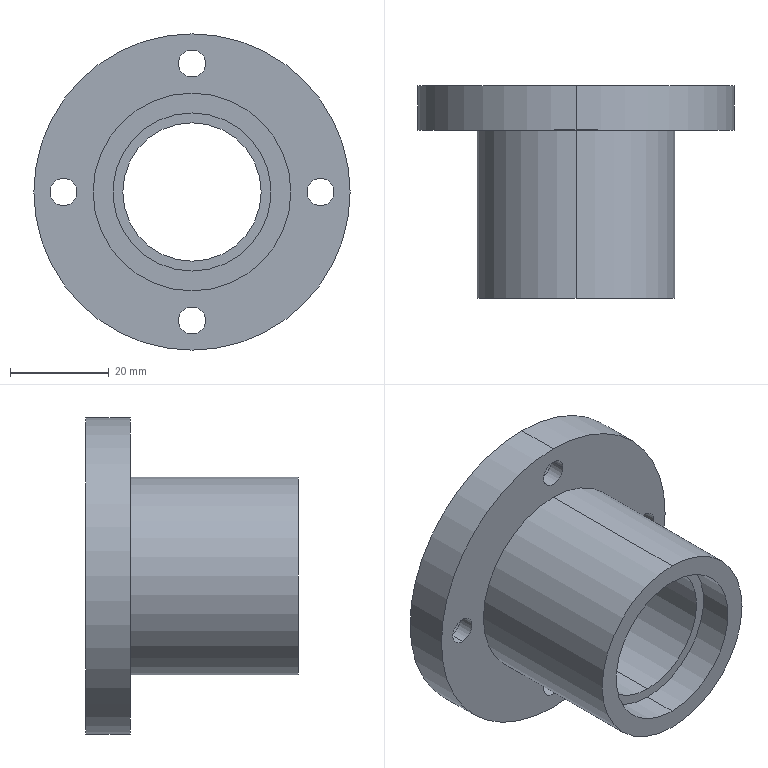Part | STEP file | PN_0011 shaft seat | 1 solid | 35 faces | box 64 x 43 x 64 mm | volume 40458 mm3 | cylinder 26 | plane 9 | commonest cylinder face diameters 5.5 x8 10 x8 32 x4 28 x2 40 x2 64 x2